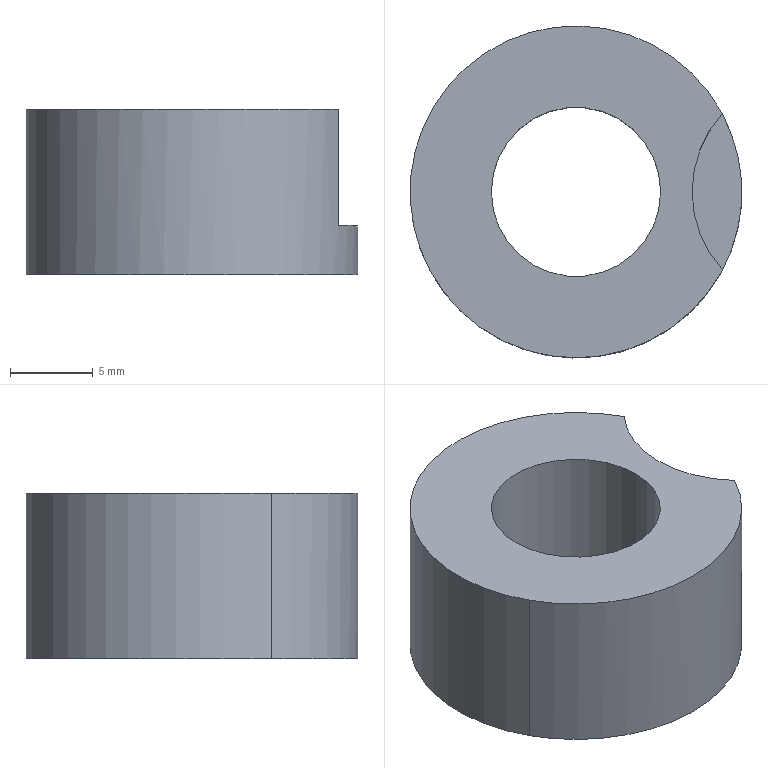Part | CATIA | 1 solid | 9 faces | box 20 x 20 x 10 mm | volume 2190 mm3 | cylinder 6 | plane 3 | commonest cylinder face diameters 10.2 x2 14 x2 20 x2
STEP:
#1=CARTESIAN_POINT('',(-8.776,-4.794,-10.));
#2=VERTEX_POINT('',#1);
#3=CARTESIAN_POINT('',(-8.776,-4.794,0.));
#4=VERTEX_POINT('',#3);
#5=CARTESIAN_POINT('',(-8.776,-4.794,-5.));
#6=DIRECTION('',(0.,0.,1.));
#7=VECTOR('',#6,1.);
#8=LINE('',#5,#7);
#9=EDGE_CURVE('',#2,#4,#8,.T.);
#10=ORIENTED_EDGE('',*,*,#9,.T.);
#11=CARTESIAN_POINT('',(8.776,4.794,0.));
#12=VERTEX_POINT('',#11);
#13=CARTESIAN_POINT('',(0.,0.,0.));
#14=DIRECTION('',(0.,0.,1.));
#15=AXIS2_PLACEMENT_3D('',#13,#14,$);
#16=CIRCLE('',#15,10.);
#17=EDGE_CURVE('',#12,#4,#16,.T.);
#18=ORIENTED_EDGE('',*,*,#17,.F.);
#19=CARTESIAN_POINT('',(8.776,4.794,-10.));
#20=VERTEX_POINT('',#19);
#21=CARTESIAN_POINT('',(8.776,4.794,-5.));
#22=DIRECTION('',(0.,0.,1.));
#23=VECTOR('',#22,1.);
#24=LINE('',#21,#23);
#25=EDGE_CURVE('',#20,#12,#24,.T.);
#26=ORIENTED_EDGE('',*,*,#25,.F.);
#27=CARTESIAN_POINT('',(0.,0.,-10.));
#28=DIRECTION('',(0.,0.,1.));
#29=AXIS2_PLACEMENT_3D('',#27,#28,$);
#30=CIRCLE('',#29,10.);
#31=EDGE_CURVE('',#20,#2,#30,.T.);
#32=ORIENTED_EDGE('',*,*,#31,.T.);
#33=EDGE_LOOP('',(#10,#18,#26,#32));
#34=FACE_OUTER_BOUND('',#33,.T.);
#35=CARTESIAN_POINT('',(0.,0.,-5.));
#36=DIRECTION('',(0.,0.,1.));
#37=DIRECTION('',(0.8776,0.4794,0.));
#38=AXIS2_PLACEMENT_3D('',#35,#36,#37);
#39=CYLINDRICAL_SURFACE('',#38,10.);
#40=ADVANCED_FACE('',(#34),#39,.T.);
#41=CARTESIAN_POINT('',(0.,0.,-10.));
#42=DIRECTION('',(0.,0.,1.));
#43=AXIS2_PLACEMENT_3D('',#41,#42,$);
#44=CIRCLE('',#43,10.);
#45=EDGE_CURVE('',#2,#20,#44,.T.);
#46=ORIENTED_EDGE('',*,*,#45,.F.);
#47=ORIENTED_EDGE('',*,*,#31,.F.);
#48=EDGE_LOOP('',(#46,#47));
#49=FACE_OUTER_BOUND('',#48,.T.);
#50=CARTESIAN_POINT('',(-5.1,0.,-10.));
#51=VERTEX_POINT('',#50);
#52=CARTESIAN_POINT('',(5.1,0.,-10.));
#53=VERTEX_POINT('',#52);
#54=CARTESIAN_POINT('',(0.,0.,-10.));
#55=DIRECTION('',(0.,0.,1.));
#56=AXIS2_PLACEMENT_3D('',#54,#55,$);
#57=CIRCLE('',#56,5.1);
#58=EDGE_CURVE('',#51,#53,#57,.T.);
#59=ORIENTED_EDGE('',*,*,#58,.T.);
#60=CARTESIAN_POINT('',(0.,0.,-10.));
#61=DIRECTION('',(0.,0.,1.));
#62=AXIS2_PLACEMENT_3D('',#60,#61,$);
#63=CIRCLE('',#62,5.1);
#64=EDGE_CURVE('',#53,#51,#63,.T.);
#65=ORIENTED_EDGE('',*,*,#64,.T.);
#66=EDGE_LOOP('',(#59,#65));
#67=FACE_BOUND('',#66,.T.);
#68=CARTESIAN_POINT('',(10.,0.,-10.));
#69=DIRECTION('',(0.,0.,1.));
#70=DIRECTION('',(1.,0.,0.));
#71=AXIS2_PLACEMENT_3D('',#68,#69,#70);
#72=PLANE('',#71);
#73=ADVANCED_FACE('',(#49,#67),#72,.F.);
#74=ORIENTED_EDGE('',*,*,#58,.F.);
#75=CARTESIAN_POINT('',(-5.1,0.,0.));
#76=VERTEX_POINT('',#75);
#77=CARTESIAN_POINT('',(-5.1,0.,-16.61));
#78=DIRECTION('',(0.,0.,-1.));
#79=VECTOR('',#78,1.);
#80=LINE('',#77,#79);
#81=EDGE_CURVE('',#76,#51,#80,.T.);
#82=ORIENTED_EDGE('',*,*,#81,.F.);
#83=CARTESIAN_POINT('',(5.1,0.,0.));
#84=VERTEX_POINT('',#83);
#85=CARTESIAN_POINT('',(0.,0.,0.));
#86=DIRECTION('',(0.,0.,-1.));
#87=AXIS2_PLACEMENT_3D('',#85,#86,$);
#88=CIRCLE('',#87,5.1);
#89=EDGE_CURVE('',#84,#76,#88,.T.);
#90=ORIENTED_EDGE('',*,*,#89,.F.);
#91=CARTESIAN_POINT('',(5.1,0.,-16.61));
#92=DIRECTION('',(0.,0.,-1.));
#93=VECTOR('',#92,1.);
#94=LINE('',#91,#93);
#95=EDGE_CURVE('',#84,#53,#94,.T.);
#96=ORIENTED_EDGE('',*,*,#95,.T.);
#97=EDGE_LOOP('',(#74,#82,#90,#96));
#98=FACE_OUTER_BOUND('',#97,.T.);
#99=CARTESIAN_POINT('',(0.,0.,-16.61));
#100=DIRECTION('',(0.,0.,-1.));
#101=DIRECTION('',(1.,0.,0.));
#102=AXIS2_PLACEMENT_3D('',#99,#100,#101);
#103=CYLINDRICAL_SURFACE('',#102,5.1);
#104=ADVANCED_FACE('',(#98),#103,.F.);
#105=ORIENTED_EDGE('',*,*,#64,.F.);
#106=ORIENTED_EDGE('',*,*,#95,.F.);
#107=CARTESIAN_POINT('',(0.,0.,0.));
#108=DIRECTION('',(0.,0.,-1.));
#109=AXIS2_PLACEMENT_3D('',#107,#108,$);
#110=CIRCLE('',#109,5.1);
#111=EDGE_CURVE('',#76,#84,#110,.T.);
#112=ORIENTED_EDGE('',*,*,#111,.F.);
#113=ORIENTED_EDGE('',*,*,#81,.T.);
#114=EDGE_LOOP('',(#105,#106,#112,#113));
#115=FACE_OUTER_BOUND('',#114,.T.);
#116=CARTESIAN_POINT('',(0.,0.,-16.61));
#117=DIRECTION('',(0.,0.,-1.));
#118=DIRECTION('',(-1.,0.,0.));
#119=AXIS2_PLACEMENT_3D('',#116,#117,#118);
#120=CYLINDRICAL_SURFACE('',#119,5.1);
#121=ADVANCED_FACE('',(#115),#120,.F.);
#122=CARTESIAN_POINT('',(8.821,4.71,0.));
#123=VERTEX_POINT('',#122);
#124=CARTESIAN_POINT('',(0.,0.,0.));
#125=DIRECTION('',(0.,0.,1.));
#126=AXIS2_PLACEMENT_3D('',#124,#125,$);
#127=CIRCLE('',#126,10.);
#128=EDGE_CURVE('',#123,#12,#127,.T.);
#129=ORIENTED_EDGE('',*,*,#128,.T.);
#130=ORIENTED_EDGE('',*,*,#17,.T.);
#131=CARTESIAN_POINT('',(8.821,-4.71,0.));
#132=VERTEX_POINT('',#131);
#133=CARTESIAN_POINT('',(0.,0.,0.));
#134=DIRECTION('',(0.,0.,1.));
#135=AXIS2_PLACEMENT_3D('',#133,#134,$);
#136=CIRCLE('',#135,10.);
#137=EDGE_CURVE('',#4,#132,#136,.T.);
#138=ORIENTED_EDGE('',*,*,#137,.T.);
#139=CARTESIAN_POINT('',(7.,0.,0.));
#140=VERTEX_POINT('',#139);
#141=CARTESIAN_POINT('',(14.,0.,0.));
#142=DIRECTION('',(0.,0.,1.));
#143=AXIS2_PLACEMENT_3D('',#141,#142,$);
#144=CIRCLE('',#143,7.);
#145=EDGE_CURVE('',#140,#132,#144,.T.);
#146=ORIENTED_EDGE('',*,*,#145,.F.);
#147=CARTESIAN_POINT('',(14.,0.,0.));
#148=DIRECTION('',(0.,0.,1.));
#149=AXIS2_PLACEMENT_3D('',#147,#148,$);
#150=CIRCLE('',#149,7.);
#151=EDGE_CURVE('',#123,#140,#150,.T.);
#152=ORIENTED_EDGE('',*,*,#151,.F.);
#153=EDGE_LOOP('',(#129,#130,#138,#146,#152));
#154=FACE_OUTER_BOUND('',#153,.T.);
#155=ORIENTED_EDGE('',*,*,#89,.T.);
#156=ORIENTED_EDGE('',*,*,#111,.T.);
#157=EDGE_LOOP('',(#155,#156));
#158=FACE_BOUND('',#157,.T.);
#159=CARTESIAN_POINT('',(0.,0.,0.));
#160=DIRECTION('',(0.,0.,1.));
#161=DIRECTION('',(1.,0.,0.));
#162=AXIS2_PLACEMENT_3D('',#159,#160,#161);
#163=PLANE('',#162);
#164=ADVANCED_FACE('',(#154,#158),#163,.T.);
#165=ORIENTED_EDGE('',*,*,#137,.F.);
#166=ORIENTED_EDGE('',*,*,#9,.F.);
#167=ORIENTED_EDGE('',*,*,#45,.T.);
#168=ORIENTED_EDGE('',*,*,#25,.T.);
#169=ORIENTED_EDGE('',*,*,#128,.F.);
#170=CARTESIAN_POINT('',(8.821,4.71,-7.));
#171=VERTEX_POINT('',#170);
#172=CARTESIAN_POINT('',(8.821,4.71,-5.));
#173=DIRECTION('',(0.,0.,1.));
#174=VECTOR('',#173,1.);
#175=LINE('',#172,#174);
#176=EDGE_CURVE('',#171,#123,#175,.T.);
#177=ORIENTED_EDGE('',*,*,#176,.F.);
#178=CARTESIAN_POINT('',(8.821,-4.71,-7.));
#179=VERTEX_POINT('',#178);
#180=CARTESIAN_POINT('',(0.,0.,-7.));
#181=DIRECTION('',(0.,0.,1.));
#182=AXIS2_PLACEMENT_3D('',#180,#181,$);
#183=CIRCLE('',#182,10.);
#184=EDGE_CURVE('',#179,#171,#183,.T.);
#185=ORIENTED_EDGE('',*,*,#184,.F.);
#186=CARTESIAN_POINT('',(8.821,-4.71,-5.));
#187=DIRECTION('',(0.,0.,1.));
#188=VECTOR('',#187,1.);
#189=LINE('',#186,#188);
#190=EDGE_CURVE('',#179,#132,#189,.T.);
#191=ORIENTED_EDGE('',*,*,#190,.T.);
#192=EDGE_LOOP('',(#165,#166,#167,#168,#169,#177,#185,#191));
#193=FACE_OUTER_BOUND('',#192,.T.);
#194=ADVANCED_FACE('',(#193),#39,.T.);
#195=CARTESIAN_POINT('',(7.,0.,-7.));
#196=VERTEX_POINT('',#195);
#197=CARTESIAN_POINT('',(14.,0.,-7.));
#198=DIRECTION('',(0.,0.,1.));
#199=AXIS2_PLACEMENT_3D('',#197,#198,$);
#200=CIRCLE('',#199,7.);
#201=EDGE_CURVE('',#171,#196,#200,.T.);
#202=ORIENTED_EDGE('',*,*,#201,.T.);
#203=CARTESIAN_POINT('',(14.,0.,-7.));
#204=DIRECTION('',(0.,0.,1.));
#205=AXIS2_PLACEMENT_3D('',#203,#204,$);
#206=CIRCLE('',#205,7.);
#207=EDGE_CURVE('',#196,#179,#206,.T.);
#208=ORIENTED_EDGE('',*,*,#207,.T.);
#209=ORIENTED_EDGE('',*,*,#184,.T.);
#210=EDGE_LOOP('',(#202,#208,#209));
#211=FACE_OUTER_BOUND('',#210,.T.);
#212=CARTESIAN_POINT('',(0.,0.,-7.));
#213=DIRECTION('',(0.,0.,1.));
#214=DIRECTION('',(1.,0.,0.));
#215=AXIS2_PLACEMENT_3D('',#212,#213,#214);
#216=PLANE('',#215);
#217=ADVANCED_FACE('',(#211),#216,.T.);
#218=ORIENTED_EDGE('',*,*,#176,.T.);
#219=ORIENTED_EDGE('',*,*,#151,.T.);
#220=CARTESIAN_POINT('',(7.,0.,-4.11));
#221=DIRECTION('',(0.,0.,1.));
#222=VECTOR('',#221,1.);
#223=LINE('',#220,#222);
#224=EDGE_CURVE('',#140,#196,#223,.F.);
#225=ORIENTED_EDGE('',*,*,#224,.T.);
#226=ORIENTED_EDGE('',*,*,#201,.F.);
#227=EDGE_LOOP('',(#218,#219,#225,#226));
#228=FACE_OUTER_BOUND('',#227,.T.);
#229=CARTESIAN_POINT('',(14.,0.,-4.11));
#230=DIRECTION('',(0.,0.,1.));
#231=DIRECTION('',(1.,0.,0.));
#232=AXIS2_PLACEMENT_3D('',#229,#230,#231);
#233=CYLINDRICAL_SURFACE('',#232,7.);
#234=ADVANCED_FACE('',(#228),#233,.F.);
#235=ORIENTED_EDGE('',*,*,#190,.F.);
#236=ORIENTED_EDGE('',*,*,#207,.F.);
#237=ORIENTED_EDGE('',*,*,#224,.F.);
#238=ORIENTED_EDGE('',*,*,#145,.T.);
#239=EDGE_LOOP('',(#235,#236,#237,#238));
#240=FACE_OUTER_BOUND('',#239,.T.);
#241=ADVANCED_FACE('',(#240),#233,.F.);
#242=CLOSED_SHELL('',(#40,#73,#104,#121,#164,#194,#217,#234,#241));
#243=MANIFOLD_SOLID_BREP('',#242);
#244=(LENGTH_UNIT()NAMED_UNIT(*)SI_UNIT(.MILLI.,.METRE.));
#245=UNCERTAINTY_MEASURE_WITH_UNIT(LENGTH_MEASURE(0.005),#244,'','');
#246=(NAMED_UNIT(*)PLANE_ANGLE_UNIT()SI_UNIT($,.RADIAN.));
#247=(NAMED_UNIT(*)SI_UNIT($,.STERADIAN.)SOLID_ANGLE_UNIT());
#248=(GEOMETRIC_REPRESENTATION_CONTEXT(3)GLOBAL_UNCERTAINTY_ASSIGNED_CONTEXT((#245))GLOBAL_UNIT_ASSIGNED_CONTEXT((#244,#246,#247))REPRESENTATION_CONTEXT('',''));
#249=ADVANCED_BREP_SHAPE_REPRESENTATION('',(#243),#248);